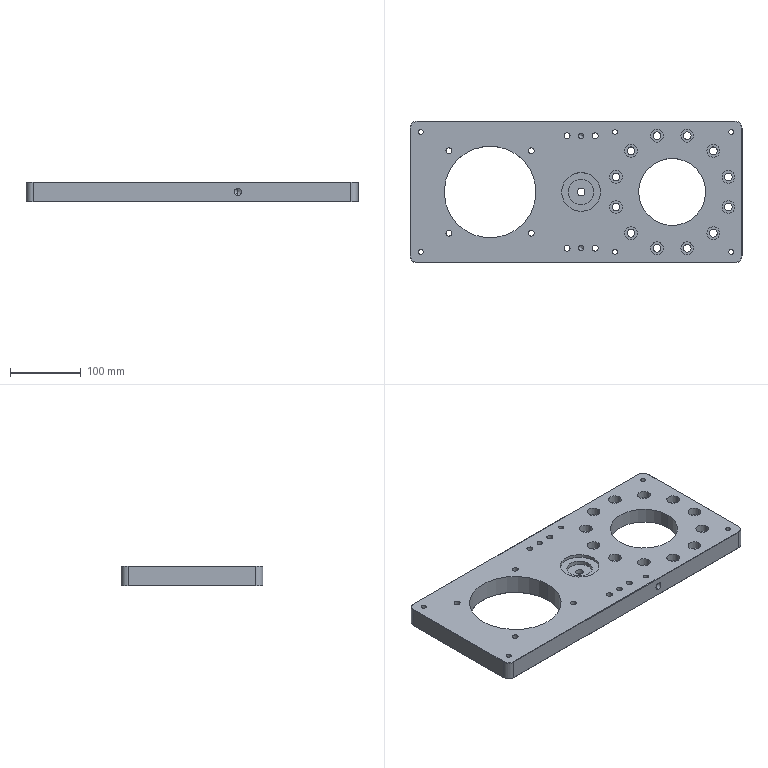Part | SolidWorks | features HoleWzd 7, ICE 7, MirrorPattern 3, Chamfer 2, Fillet 2, CirPattern 1, Extrusion 1 | 1 solid | 162 faces | box 470.5 x 201 x 28 mm | volume 1919904 mm3 | cylinder 102 | cone 30 | plane 30 | commonest cylinder face diameters 11 x26 18 x26 8.5 x16 6.8 x12 8 x4 10.2 x4